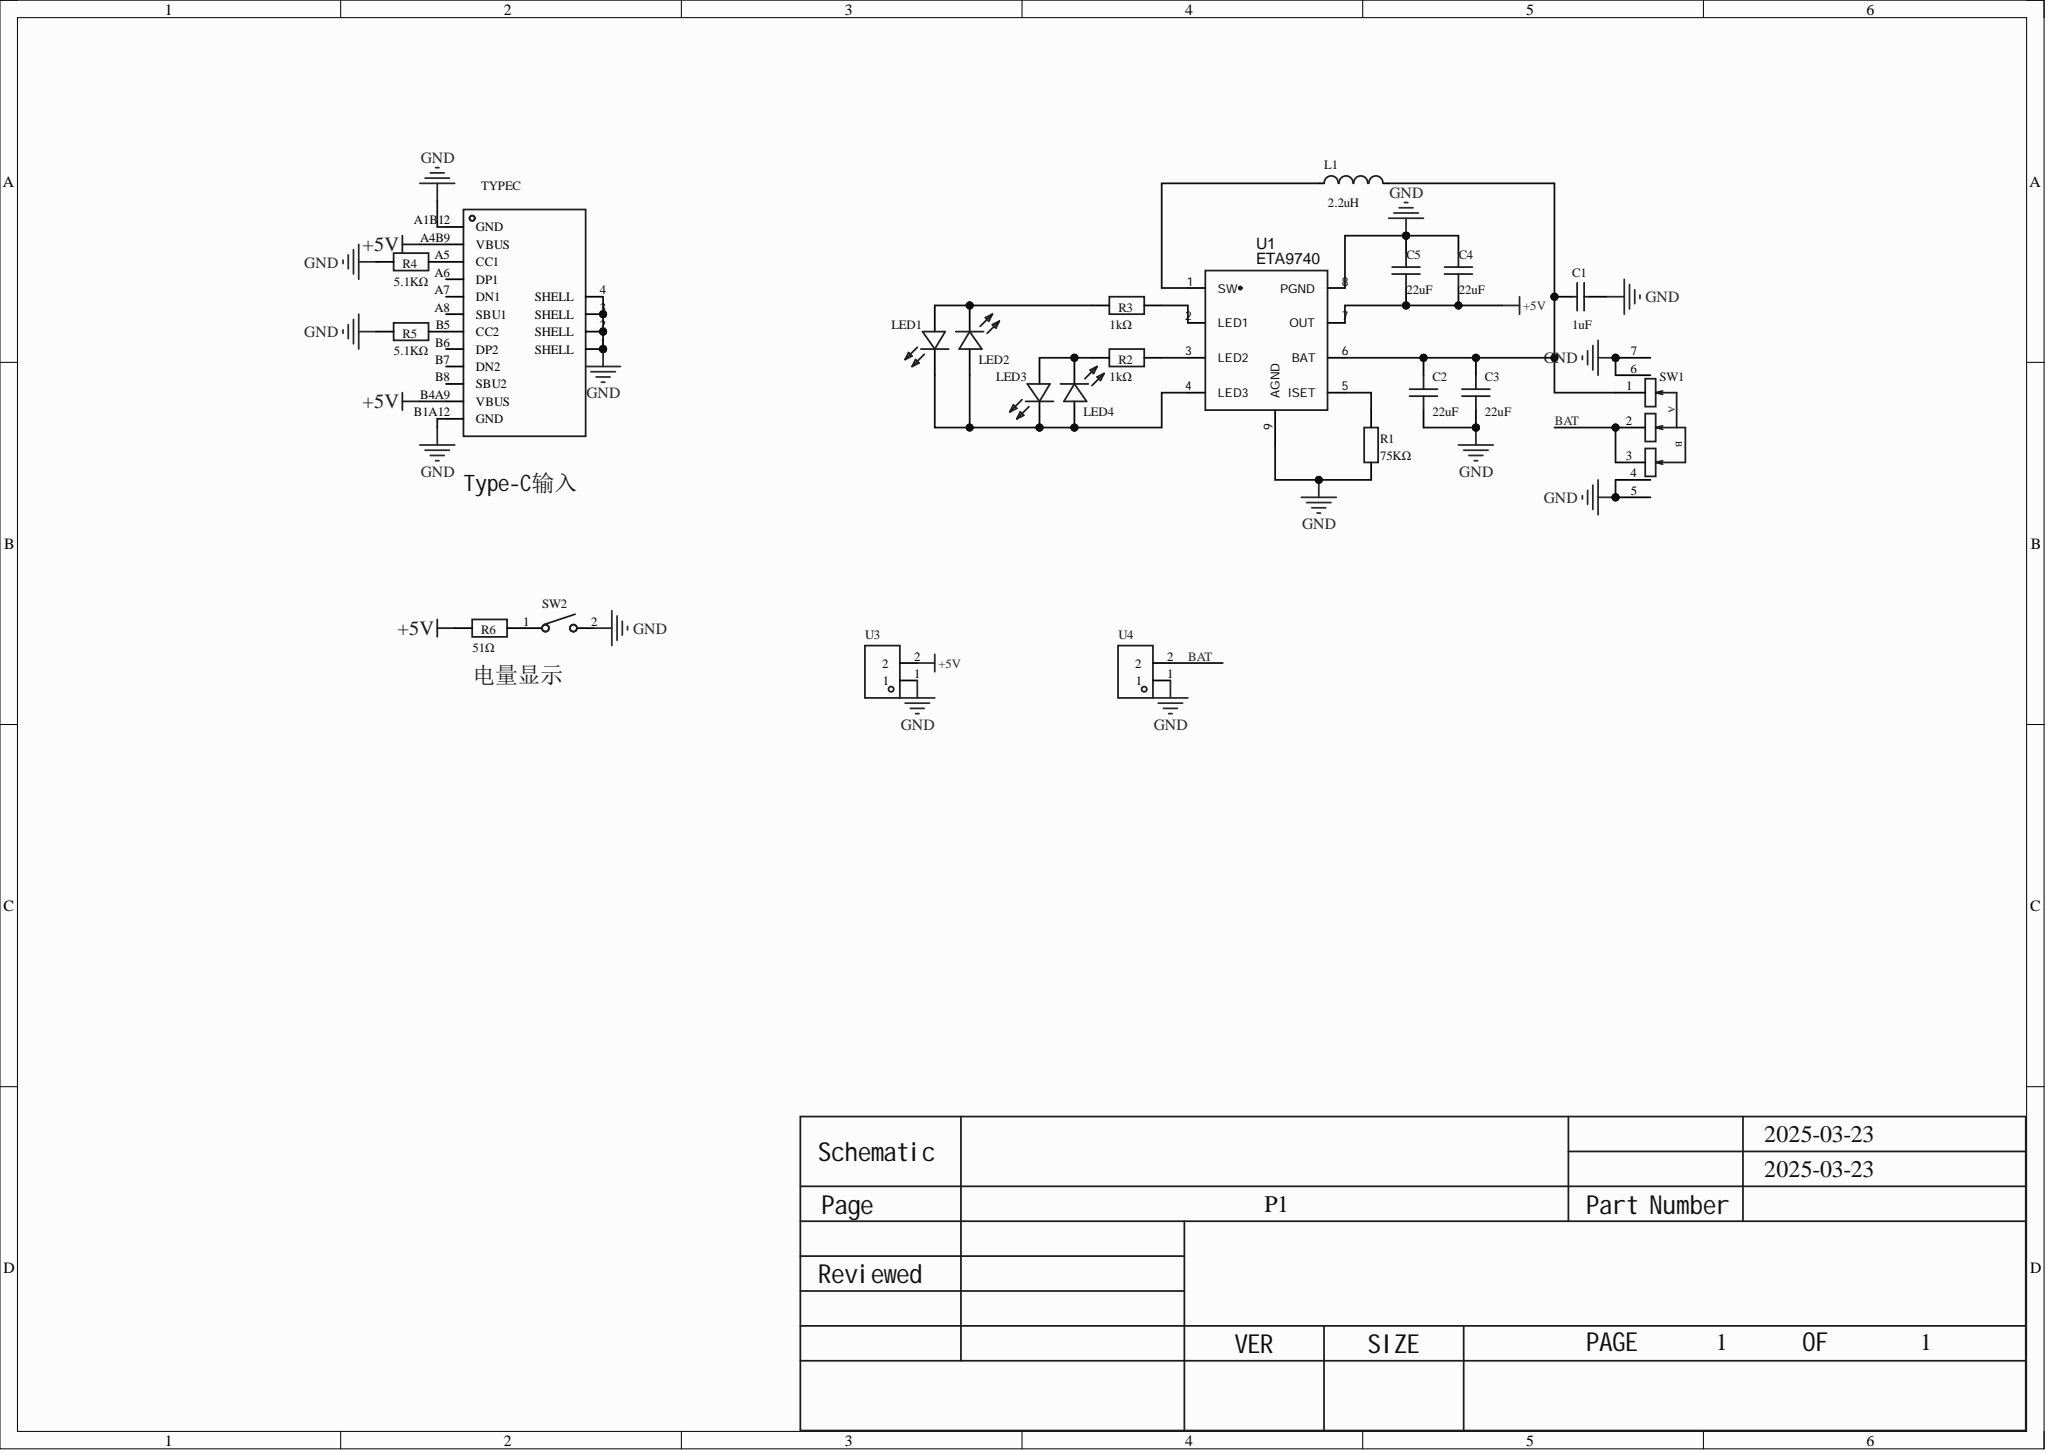Circuit board | Altium Designer | 22 parts | 14 nets
Bill of materials:
Comment,Description,Designator,Footprint,LibRef,Quantity
"CL21B105KBFNNNE","","C1","C0805","CL21B105KBFNNNE","1"
"CL21A226MAQNNNE_C45783","","C2, C3, C4, C5","C0805","CL21A226MAQNNNE_C45783","4"
"YTA0520-2R2M","","L1","IND-SMD_L5.4-W5.2","YTA0520-2R2M","1"
"led0805","","LED1, LED2, LED3, LED4","LED0805-RD","led0805","4"
"AC0805JR-07100KL","","R1","R0805","AC0805JR-07100KL","1"
"RT0805CRE071KL","","R2, R3, R4, R5, R6","R0805","RT0805CRE071KL","5"
"MK-12C02-G015","","SW1","SW-SMD_G-SWITCH_MK-12C02-G015","MK-12C02-G015","1"
"ST-1185U","","SW2","SW-SMD_ST-1185U","ST-1185U","1"
"TYPE-C 16PIN 3MD(385)","","TYPEC","USB-C-SMD_TYPE-C16PIN","TYPE-C 16PIN 3MD(385)","1"
"ETA9740","","U1","ESOP-8","ETA9740","1"
"2.54-1*2","","U3, U4","HDR-TH_2P-P2.54-V-M","2.54-1*2","2"
Netlist (Protel format):
[
C1
C0805
CL21B105KBFNNNE



]
[
C2
C0805
CL21A226MAQNNNE_C45783



]
[
C3
C0805
CL21A226MAQNNNE_C45783



]
[
C4
C0805
CL21A226MAQNNNE_C45783



]
[
C5
C0805
CL21A226MAQNNNE_C45783



]
[
L1
IND-SMD_L5.4-W5.2
YTA0520-2R2M



]
[
LED1
LED0805-RD
led0805



]
[
LED2
LED0805-RD
led0805



]
[
LED3
LED0805-RD
led0805



]
[
LED4
LED0805-RD
led0805



]
[
R1
R0805
AC0805JR-07100KL



]
[
R2
R0805
RT0805CRE071KL



]
[
R3
R0805
RT0805CRE071KL



]
[
R4
R0805
RT0805CRE071KL



]
[
R5
R0805
RT0805CRE071KL



]
[
R6
R0805
RT0805CRE071KL



]
[
SW1
SW-SMD_G-SWITCH_MK-12C02-G015
MK-12C02-G015



]
[
SW2
SW-SMD_ST-1185U
ST-1185U



]
[
TYPEC
USB-C-SMD_TYPE-C16PIN
TYPE-C 16PIN 3MD(385)



]
[
U1
ESOP-8
ETA9740



]
[
U3
HDR-TH_2P-P2.54-V-M
2.54-1*2



]
[
U4
HDR-TH_2P-P2.54-V-M
2.54-1*2



]
(
NetR6_2
R6-2
SW2-1
)
(
NetR5_2
R5-2
TYPEC-B5
)
(
NetR4_2
R4-2
TYPEC-A5
)
(
NetR3_2
R3-2
U1-2
)
(
NetR2_2
R2-2
U1-3
)
(
NetR1_2
R1-2
U1-5
)
(
NetLED3_2
LED3-2
LED4-1
R2-1
)
(
NetLED1_2
LED1-2
LED2-1
R3-1
)
(
NetLED1_1
LED1-1
LED2-2
LED3-1
LED4-2
U1-4
)
(
NetL1_1
L1-1
U1-1
)
(
NetC1_1
C1-1
C2-2
C3-2
L1-2
SW1-1
U1-6
)
(
GND
C1-2
C2-1
C3-1
C4-1
C5-1
R1-1
R4-1
R5-1
SW1-4
SW1-5
SW1-6
SW1-7
SW2-2
TYPEC-1
TYPEC-2
TYPEC-3
TYPEC-4
TYPEC-A1B12
TYPEC-B1A12
U1-8
U1-9
U3-1
U4-1
)
(
BAT
SW1-2
SW1-3
U4-2
)
(
+5V
C4-2
C5-2
R6-1
TYPEC-A4B9
TYPEC-B4A9
U1-7
U3-2
)